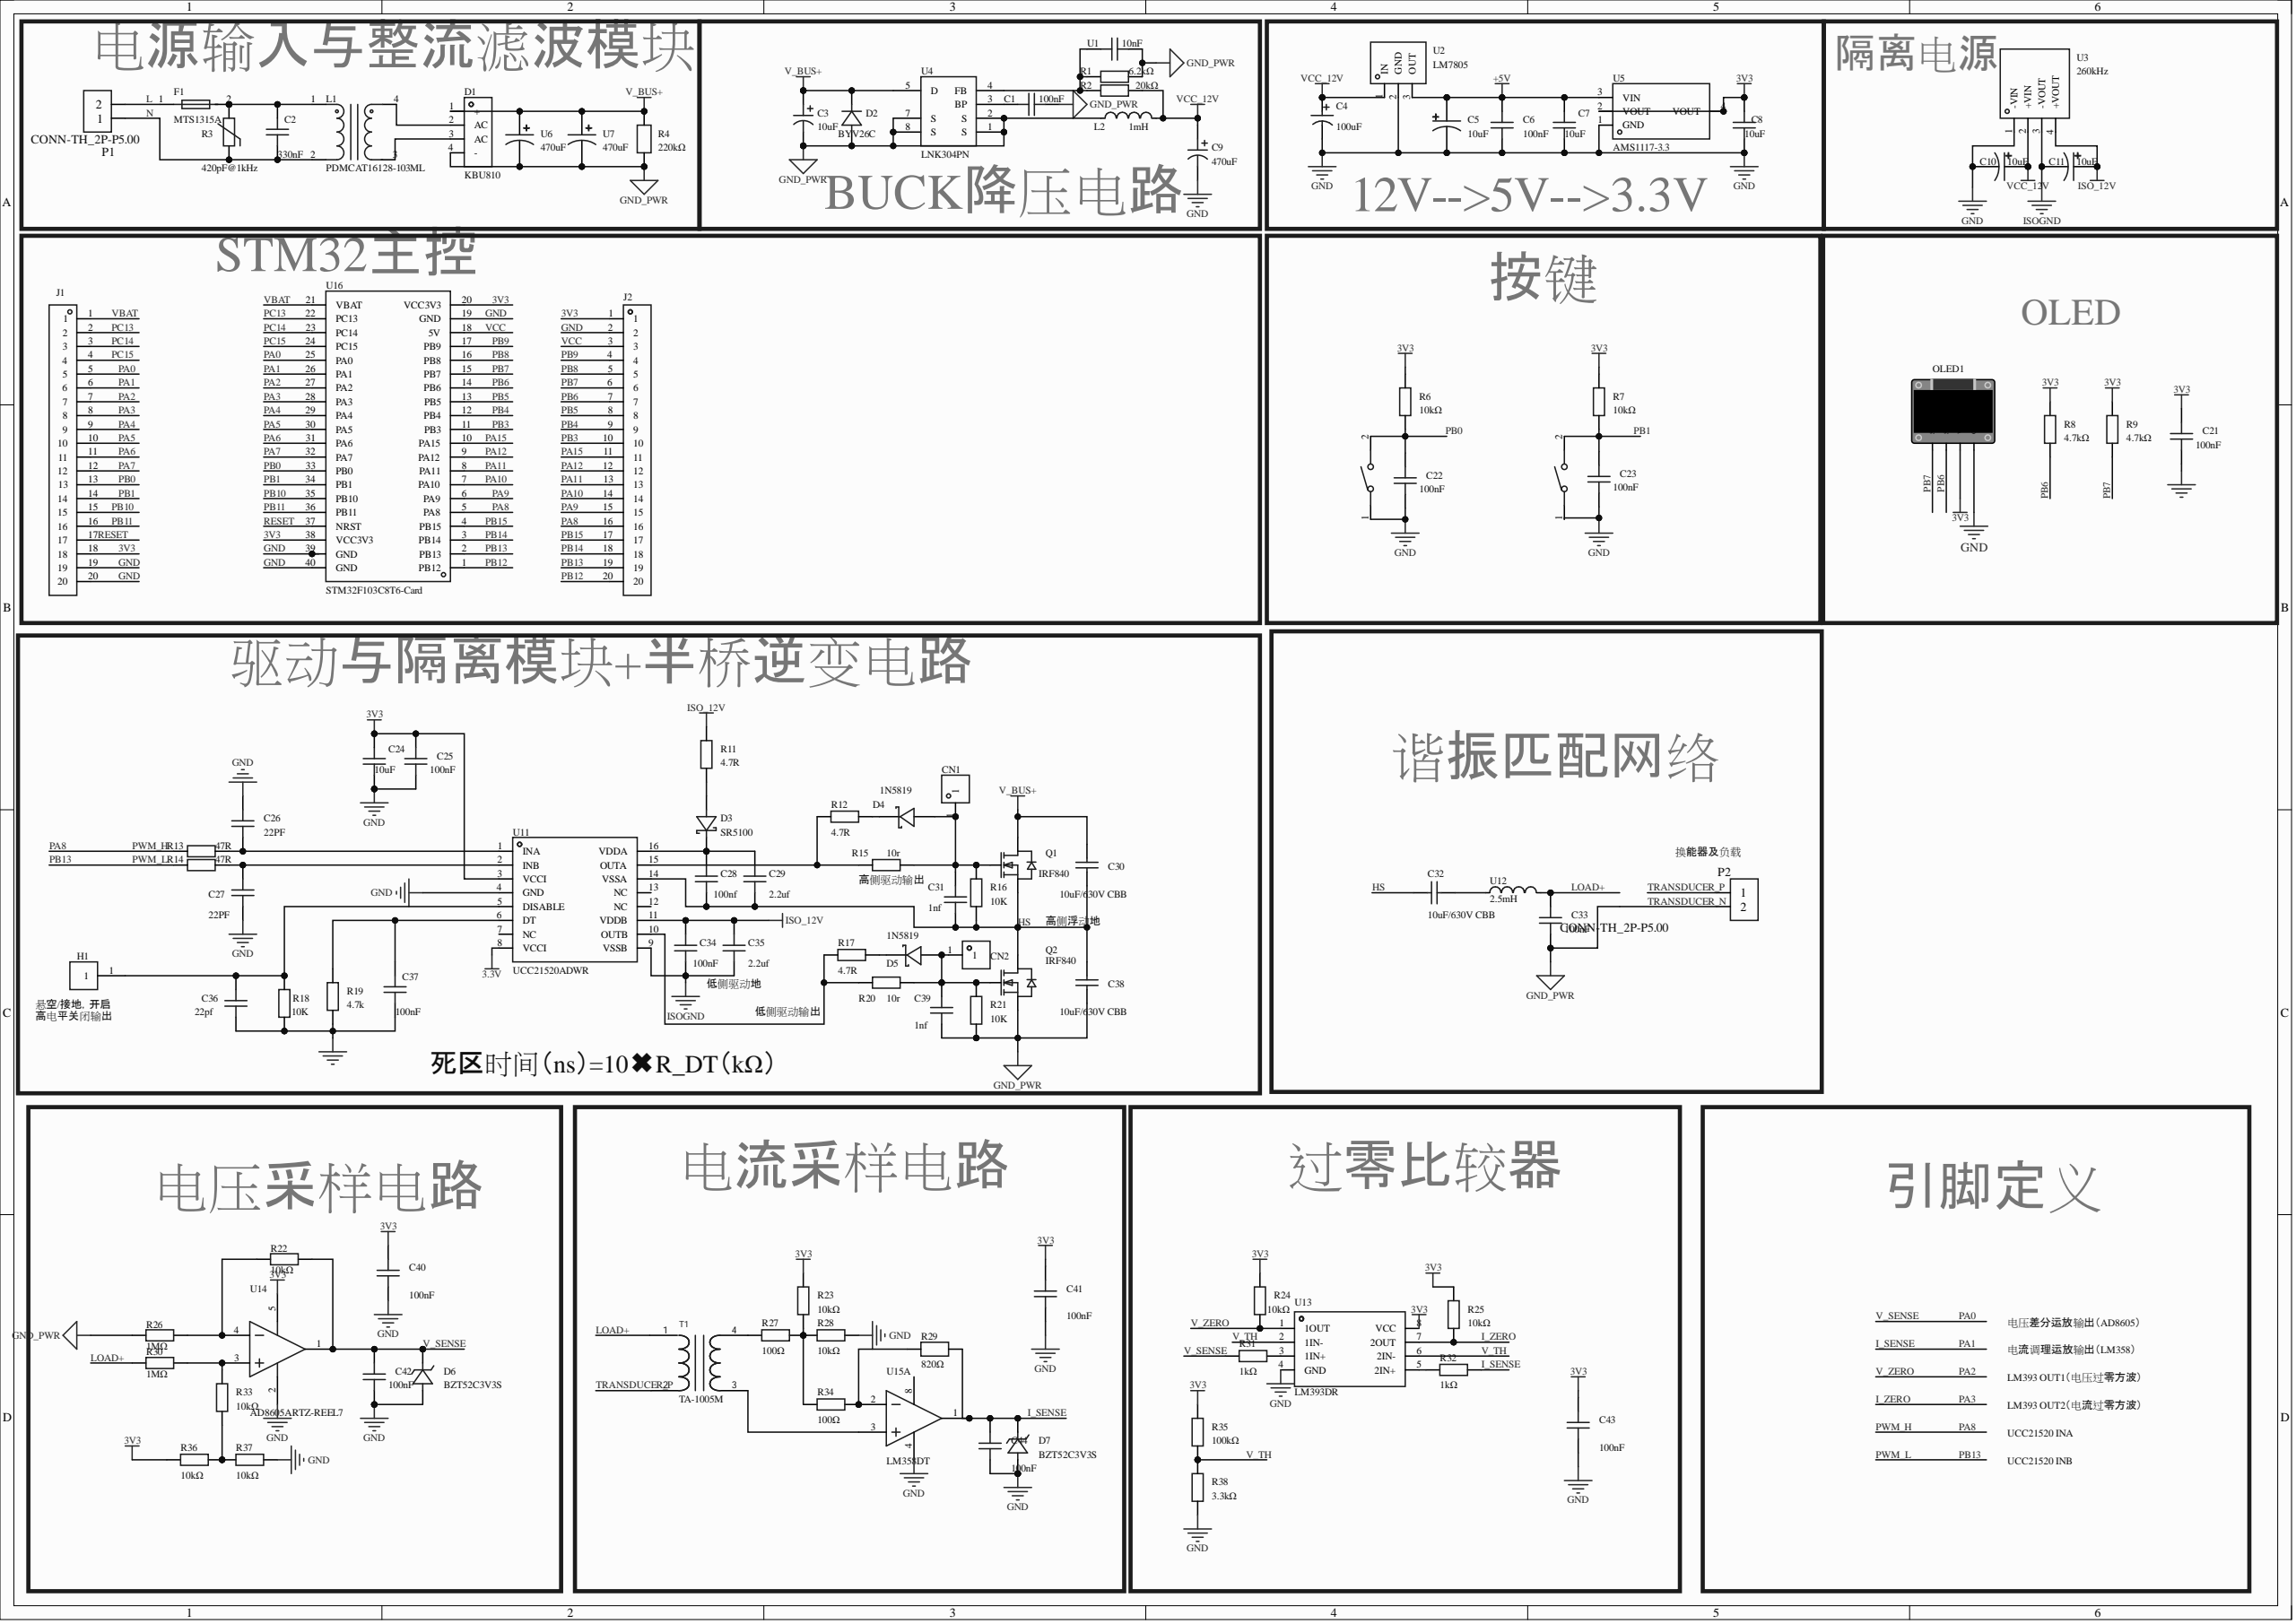Circuit board | Altium Designer | 107 parts | 76 nets
Bill of materials:
Comment,Description,Designator,Footprint,LibRef,Quantity
"100nF","","C1, C6","CAP-TH_L5.0-W2.5-P5.00-D1.0","CC1H104MC1FD3F6C10MF","2"
"330nF","","C2","CAP-TH_L18.0-W7.0-P15.00-D0.7","MKP62-275VAC/334","1"
"10uF","","C3","CAP-TH_BD10.0-P5.00-D0.6-FD_1","ERG450V10M10x16","1"
"100uF","","C4","CAP-SMD_BD6.3-L6.6-W6.6-FD","RVT1E101M0607_C72477","1"
"10uF","","C5","CAP-SMD_BD4.0-L4.3-W4.3-FD","VT1C100M0405","1"
"10uF","","C7, C8, C24","C0805","C0805X106K010T","3"
"470uF","","C9","CAP-SMD_BD8.0-L8.3-W8.3-LS9.2-FD-H10.5","RV35V470M8X10","1"
"10uF","","C10, C11","CAP-SMD_BD4.0-L4.3-W4.3-FD_1","VT1E100M0405","2"
"100nF","","C21, C22, C23, C25, C33, C40, C41, C42, C43, C44","C0603","CC0603KRX7R9BB104_1","10"
"22PF","","C26, C27, C36","C0805","CAP_0805","3"
"100nf","","C28, C34, C37","C0805","CAP_0805","3"
"2.2uf","","C29, C35","C0805","CAP_0805","2"
"10uF/630V CBB","","C30, C32, C38","1uf/630V CBB","1uF/630V CBB","3"
"1nf","","C31, C39","C0805","CAP_0805","2"
"RH-5001","","CN1, CN2","TEST-TH_BD2.54-P1.4_BLACK","RH-5001","2"
"KBU810","","D1","DIO-BG-TH_L23.2-W6.8-P5.10_KBU","KBU810_C34835","1"
"BYV26C","","D2","DO-41_BD2.6-L5.1-P9.00-D0.8-RD","BYV26C","1"
"SR5100","","D3","DO-201AD_BD5.3-L8.4-P12.50-D1.4-RD","SR5100_C784810","1"
"1N5819","","D4, D5","DO-41_BD2.4-L4.7-P8.70-D0.9-FD","1N5819_C110032","2"
"BZT52C3V3S","","D6, D7","SOD-323_L1.7-W1.3-LS2.6-RD","BZT52C3V3S_C19077437","2"
"MTS1315A","","F1","FUSE-TH_L8.4-W4.0-P5.08-D0.6","MTS1315A","1"
"PZ254V-11-01P","","H1","HDR-TH_1P-P2.54-V-M","PZ254V-11-01P","1"
"2.54-1*20P直针","","J1, J2","HDR-TH_20P-P2.54-V-M-1","2.54-1*20P直针","2"
"PDMCAT16128-103ML","","L1","IND-TH_4P-L20.0-W12.0-P6.00-LS10.0-BL","PDMCAT16128-103ML","1"
"1mH","","L2","IND-TH_BD8.5-P5.00-D0.6","SLP0810R-102MTT","1"
"","","OLED1","0.96OLED_4P","0.96OLED模块_4P","1"
"CONN-TH_2P-P5.00","","P1, P2","CONN-TH_2P-P5.00","CONN-TH_2P-P5.00","2"
"IRF840","","Q1, Q2","TO-220-3_L10.2-W4.5-P2.54-L-1","IRF840_C2980294","2"
"6.2kΩ","","R1","R0603","0603WAF6201T5E","1"
"20kΩ","","R2","R0603","0603WAF2002T5E","1"
"420pF@1kHz","","R3","RES-TH_L15.5-W5.6-P7.50-D0.8-S1.90","14D471K_C49069733","1"
"220kΩ","","R4","RES-TH_BD3.9-L9.0-P13.00-D0.8","FMP200JR-52-220K","1"
"10kΩ","","R6, R7","R0603_1","0603WAF1002T5E","2"
"4.7kΩ","","R8, R9","R0603","0603WAF4701T5E","2"
"4.7R","","R11, R12, R17","R0805","Res_0805","3"
"47R","","R13, R14","R0805","Res_0805","2"
"10r","","R15, R20","R0805","Res_0805","2"
"10K","","R16, R18, R21","R0805","Res_0805","3"
"4.7k","","R19","R0805","Res_0805","1"
"10kΩ","","R22, R23, R24, R25, R28, R33, R36, R37","R0805","0805W8F1002T5E_C17414","8"
"1MΩ","","R26, R30","R1206","1206W4F1004T5E","2"
"100Ω","","R27, R34","R0805","0805W8F1000T5E","2"
"820Ω","","R29","R0805","FRC0805J821 TS","1"
"1kΩ","","R31, R32","R0603","1kΩ","2"
"100kΩ","","R35","R0603","100kΩ","1"
"3.3kΩ","","R38","R0603_NEW","0603WAF3301T5E","1"
"TS-1088-AR02016","","SW2, SW3","SW-SMD_L3.9-W3.0-P4.45","TS-1088-AR02016","2"
"TA-1005M","","T1","TA-1005M","TA-1005M","1"
"10nF","","U1","CAP-TH_L5.0-W2.5-P2.50-D0.5","CC1H103ZA1ED3F4D1100","1"
"LM7805","","U2","TO-220-3_L10.0-W4.5-P2.54-L","LM7805_C845394","1"
"260kHz","","U3","PWRM-TH_4P-L11.5-W6.0-P2.54_B1503S","B1205S-1WR3_C5365649","1"
"LNK304PN","","U4","DIP-8_7P-L9.7-W6.4-P2.54-LS7.6-BL-PE6","LNK304PN","1"
"AMS1117-3.3","","U5","SOT-223-3_L6.5-W3.4-P2.30-LS7.0-BR","AMS1117-3.3_C6186","1"
"470uF","","U6, U7","CAP-TH_BD35.0-P10.00-D1.5-FD","152EC0566","2"
"UCC21520ADWR","","U11","SOIC-16_L10.3-W7.5-P1.27-LS10.3-BL","UCC21520ADWR","1"
"2.5mH","","U12","IND-TH_BD9.5-P5.00-D0.7","XR8*10-252K-S","1"
"LM393DR","","U13","SOIC-8_L5.0-W4.0-P1.27-LS6.0-BL","LM393DR","1"
"AD8605ARTZ-REEL7","","U14","SOT-23-5_L3.0-W1.7-P0.95-LS2.8-BR","AD8605ARTZ-REEL7","1"
"LM358DT","","U15","SOIC-8_L4.9-W3.9-P1.27-LS6.0-BL","LM358DT","1"
"STM32F103C8T6-Card","","U16","CONN-TH_L53.3-W22.9_STM32F103C8T6-CARD","STM32F103C8T6-Card","1"
Netlist (Protel format):
[
C1
CAP-TH_L5.0-W2.5-P5.00-D1.0
100nF



]
[
C2
CAP-TH_L18.0-W7.0-P15.00-D0.7
330nF



]
[
C3
CAP-TH_BD10.0-P5.00-D0.6-FD_1
10uF



]
[
C4
CAP-SMD_BD6.3-L6.6-W6.6-FD
100uF



]
[
C5
CAP-SMD_BD4.0-L4.3-W4.3-FD
10uF



]
[
C6
CAP-TH_L5.0-W2.5-P5.00-D1.0
100nF



]
[
C7
C0805
10uF



]
[
C8
C0805
10uF



]
[
C9
CAP-SMD_BD8.0-L8.3-W8.3-LS9.2-FD-H10.5
470uF



]
[
C10
CAP-SMD_BD4.0-L4.3-W4.3-FD_1
10uF



]
[
C11
CAP-SMD_BD4.0-L4.3-W4.3-FD_1
10uF



]
[
C21
C0603
100nF



]
[
C22
C0603
100nF



]
[
C23
C0603
100nF



]
[
C24
C0805
10uF



]
[
C25
C0603
100nF



]
[
C26
C0805
22PF



]
[
C27
C0805
22PF



]
[
C28
C0805
100nf



]
[
C29
C0805
2.2uf



]
[
C30
1uf/630V CBB
10uF/630V CBB



]
[
C31
C0805
1nf



]
[
C32
1uf/630V CBB
10uF/630V CBB



]
[
C33
C0603
100nF



]
[
C34
C0805
100nF



]
[
C35
C0805
2.2uf



]
[
C36
C0805
22pf



]
[
C37
C0805
100nF



]
[
C38
1uf/630V CBB
10uF/630V CBB



]
[
C39
C0805
1nf



]
[
C40
C0603
100nF



]
[
C41
C0603
100nF



]
[
C42
C0603
100nF



]
[
C43
C0603
100nF



]
[
C44
C0603
100nF



]
[
CN1
TEST-TH_BD2.54-P1.4_BLACK
RH-5001



]
[
CN2
TEST-TH_BD2.54-P1.4_BLACK
RH-5001



]
[
D1
DIO-BG-TH_L23.2-W6.8-P5.10_KBU
KBU810



]
[
D2
DO-41_BD2.6-L5.1-P9.00-D0.8-RD
BYV26C



]
[
D3
DO-201AD_BD5.3-L8.4-P12.50-D1.4-RD
SR5100



]
[
D4
DO-41_BD2.4-L4.7-P8.70-D0.9-FD
1N5819



]
[
D5
DO-41_BD2.4-L4.7-P8.70-D0.9-FD
1N5819



]
[
D6
SOD-323_L1.7-W1.3-LS2.6-RD
BZT52C3V3S



]
[
D7
SOD-323_L1.7-W1.3-LS2.6-RD
BZT52C3V3S



]
[
F1
FUSE-TH_L8.4-W4.0-P5.08-D0.6
MTS1315A



]
[
H1
HDR-TH_1P-P2.54-V-M
PZ254V-11-01P



]
[
J1
HDR-TH_20P-P2.54-V-M-1
2.54-1*20P直针



]
[
J2
HDR-TH_20P-P2.54-V-M-1
2.54-1*20P直针



]
[
L1
IND-TH_4P-L20.0-W12.0-P6.00-LS10.0-BL
PDMCAT16128-103ML



]
[
L2
IND-TH_BD8.5-P5.00-D0.6
1mH



]
[
OLED1
0.96OLED_4P




]
[
P1
CONN-TH_2P-P5.00
CONN-TH_2P-P5.00



]
[
P2
CONN-TH_2P-P5.00
CONN-TH_2P-P5.00



]
[
Q1
TO-220-3_L10.2-W4.5-P2.54-L-1
IRF840



]
[
Q2
TO-220-3_L10.2-W4.5-P2.54-L-1
IRF840



]
[
R1
R0603
6.2kΩ



]
[
R2
R0603
20kΩ



]
[
R3
RES-TH_L15.5-W5.6-P7.50-D0.8-S1.90
420pF@1kHz



]
[
R4
RES-TH_BD3.9-L9.0-P13.00-D0.8
220kΩ



]
[
R6
R0603_1
10kΩ



]
[
R7
R0603_1
10kΩ



]
[
R8
R0603
4.7kΩ



]
[
R9
R0603
4.7kΩ



]
[
R11
R0805
4.7R



]
[
R12
R0805
4.7R



]
[
R13
R0805
47R



]
[
R14
R0805
47R



]
[
R15
R0805
10r



]
[
R16
R0805
10K



]
[
R17
R0805
4.7R



]
[
R18
R0805
10K



]
[
R19
R0805
4.7k



]
[
R20
R0805
10r



]
[
R21
R0805
10K



]
[
R22
R0805
10kΩ



]
[
R23
R0805
10kΩ



]
[
R24
R0805
10kΩ



]
[
R25
R0805
10kΩ



]
[
R26
R1206
1MΩ



]
[
R27
R0805
100Ω



]
[
R28
R0805
10kΩ



]
[
R29
R0805
820Ω



]
[
R30
R1206
1MΩ



]
[
R31
R0603
1kΩ



]
[
R32
R0603
1kΩ



]
[
R33
R0805
10kΩ



]
[
R34
R0805
100Ω



]
[
R35
R0603
100kΩ



]
[
R36
R0805
10kΩ



]
[
R37
R0805
10kΩ



]
[
R38
R0603_NEW
3.3kΩ



]
[
SW2
SW-SMD_L3.9-W3.0-P4.45
TS-1088-AR02016



]
[
SW3
SW-SMD_L3.9-W3.0-P4.45
TS-1088-AR02016



]
[
T1
TA-1005M
TA-1005M



]
[
U1
CAP-TH_L5.0-W2.5-P2.50-D0.5
10nF



]
[
U2
TO-220-3_L10.0-W4.5-P2.54-L
LM7805



]
[
U3
PWRM-TH_4P-L11.5-W6.0-P2.54_B1503S
260kHz



]
[
U4
DIP-8_7P-L9.7-W6.4-P2.54-LS7.6-BL-PE6
LNK304PN



]
[
U5
SOT-223-3_L6.5-W3.4-P2.30-LS7.0-BR
AMS1117-3.3



]
[
U6
CAP-TH_BD35.0-P10.00-D1.5-FD
470uF



]
[
U7
CAP-TH_BD35.0-P10.00-D1.5-FD
470uF



]
[
U11
SOIC-16_L10.3-W7.5-P1.27-LS10.3-BL
UCC21520ADWR



]
[
U12
IND-TH_BD9.5-P5.00-D0.7
2.5mH



]
[
U13
SOIC-8_L5.0-W4.0-P1.27-LS6.0-BL
LM393DR



]
[
U14
SOT-23-5_L3.0-W1.7-P0.95-LS2.8-BR
AD8605ARTZ-REEL7



]
[
U15
SOIC-8_L4.9-W3.9-P1.27-LS6.0-BL
LM358DT



]
[
U16
CONN-TH_L53.3-W22.9_STM32F103C8T6-CARD
STM32F103C8T6-Card



]
(
VCC_12V
C4-1
C9-1
C10-1
L2-2
R2-1
U2-1
U3-2
)
(
VCC
J2-3
U16-18
)
(
VBAT
J1-1
U16-21
)
(
V_TH
R35-1
R38-2
U13-2
U13-6
)
(
V_BUS+
C3-1
C30-1
D1-1
D2-1
Q1-2
R4-2
U4-5
U6-1
U7-1
)
(
TRANSDUCER_P
P2-1
T1-2
)
(
TRANSDUCER_N
C1-1
C3-2
C33-1
C38-2
C39-1
D1-4
D2-2
L2-1
P2-2
Q2-3
R1-1
R4-1
R21-1
R26-1
U1-1
U4-1
U4-2
U4-7
U4-8
U6-2
U7-2
)
(
RESET
J1-17
U16-37
)
(
PC15
J1-4
U16-24
)
(
PC14
J1-3
U16-23
)
(
PC13
J1-2
U16-22
)
(
PB15
J2-17
U16-4
)
(
PB14
J2-18
U16-3
)
(
PB13
J2-19
R14-1
U16-2
)
(
PB12
J2-20
U16-1
)
(
PB11
J1-16
U16-36
)
(
PB10
J1-15
U16-35
)
(
PB9
J2-4
U16-17
)
(
PB8
J2-5
U16-16
)
(
PB7
J2-6
OLED1-4
R9-1
U16-15
)
(
PB6
J2-7
OLED1-3
R8-1
U16-14
)
(
PB5
J2-8
U16-13
)
(
PB4
J2-9
U16-12
)
(
PB3
J2-10
U16-11
)
(
PB1
C23-2
J1-14
R7-1
SW3-2
U16-34
)
(
PB0
C22-2
J1-13
R6-1
SW2-2
U16-33
)
(
PA15
J2-11
U16-10
)
(
PA12
J2-12
U16-9
)
(
PA11
J2-13
U16-8
)
(
PA10
J2-14
U16-7
)
(
PA9
J2-15
U16-6
)
(
PA8
J2-16
R13-1
U16-5
)
(
PA7
J1-12
U16-32
)
(
PA6
J1-11
U16-31
)
(
PA5
J1-10
U16-30
)
(
PA4
J1-9
U16-29
)
(
PA2
J1-7
R24-2
U13-1
U16-27
)
(
PA0
C42-2
D6-1
J1-5
R22-2
R31-1
U14-1
U16-25
)
(
NetT1_3
T1-3
U15-3
)
(
NetR33_1
R33-1
R36-1
R37-2
)
(
NetR32_1
R32-1
U13-5
)
(
NetR31_2
R31-2
U13-3
)
(
NetR30_2
R30-2
R33-2
U14-3
)
(
NetR29_2
R29-2
R34-1
U15-2
)
(
NetR27_1
R27-1
T1-4
)
(
NetR23_2
R23-2
R27-2
R28-1
R34-2
)
(
NetR22_1
R22-1
R26-2
U14-4
)
(
NetR17_1
R17-1
R20-2
U11-10
)
(
NetR12_1
R12-1
R15-2
U11-15
)
(
NetR1_2
R1-2
R2-2
U1-2
U4-4
)
(
NetD5_2
D5-2
R17-2
)
(
NetD4_2
D4-2
R12-2
)
(
NetD3_2
D3-2
R11-2
)
(
NetD1_3
D1-3
L1-3
)
(
NetD1_2
D1-2
L1-4
)
(
NetC39_2
C39-2
CN2-1
D5-1
Q2-1
R20-1
R21-2
)
(
NetC37_2
C37-2
R19-2
U11-6
)
(
NetC36_2
C36-2
H1-1
R18-2
U11-5
)
(
NetC32_2
C32-2
U12-1
)
(
NetC31_2
C31-2
CN1-1
D4-1
Q1-1
R15-1
R16-2
)
(
NetC28_1
C28-1
C29-1
D3-1
U11-16
)
(
NetC27_2
C27-2
R14-2
U11-2
)
(
NetC26_1
C26-1
R13-2
U11-1
)
(
NetC2_2
C2-2
F1-2
L1-1
R3-2
)
(
NetC1_2
C1-2
U4-3
)
(
N
C2-1
L1-2
P1-1
R3-1
)
(
LOAD+
C33-2
R30-1
T1-1
U12-2
)
(
L
F1-1
P1-2
)
(
ISOGND
C11-2
C34-2
C35-2
U3-3
U11-9
)
(
ISO_12V
C11-1
C34-1
C35-1
R11-1
U3-4
U11-11
)
(
I_ZERO
J1-8
R25-2
U13-7
U16-28
)
(
I_SENSE
C44-1
D7-1
J1-6
R29-1
R32-2
U15-1
U16-26
)
(
HS
C28-2
C29-2
C30-2
C31-1
C32-1
C38-1
Q1-3
Q2-2
R16-1
U11-14
)
(
GND
C4-2
C5-2
C6-1
C7-1
C8-1
C9-2
C10-2
C21-1
C22-1
C23-1
C24-1
C25-1
C26-2
C27-1
C36-1
C37-1
C40-2
C41-2
C42-1
C43-2
C44-2
D6-2
D7-2
J1-19
J1-20
J2-2
OLED1-1
R18-1
R19-1
R28-2
R37-1
R38-1
SW2-1
SW3-1
U2-2
U3-1
U5-1
U11-4
U13-4
U14-2
U15-4
U16-19
U16-39
U16-40
)
(
+5V
C5-1
C6-2
C7-2
U2-3
U5-3
)
(
3V3
C8-2
C21-2
C24-2
C25-2
C40-1
C41-1
C43-1
J1-18
J2-1
OLED1-2
R6-2
R7-2
R8-2
R9-2
R23-1
R24-1
R25-1
R35-2
R36-2
U5-2
U5-4
U11-3
U13-8
U14-5
U16-20
U16-38
)